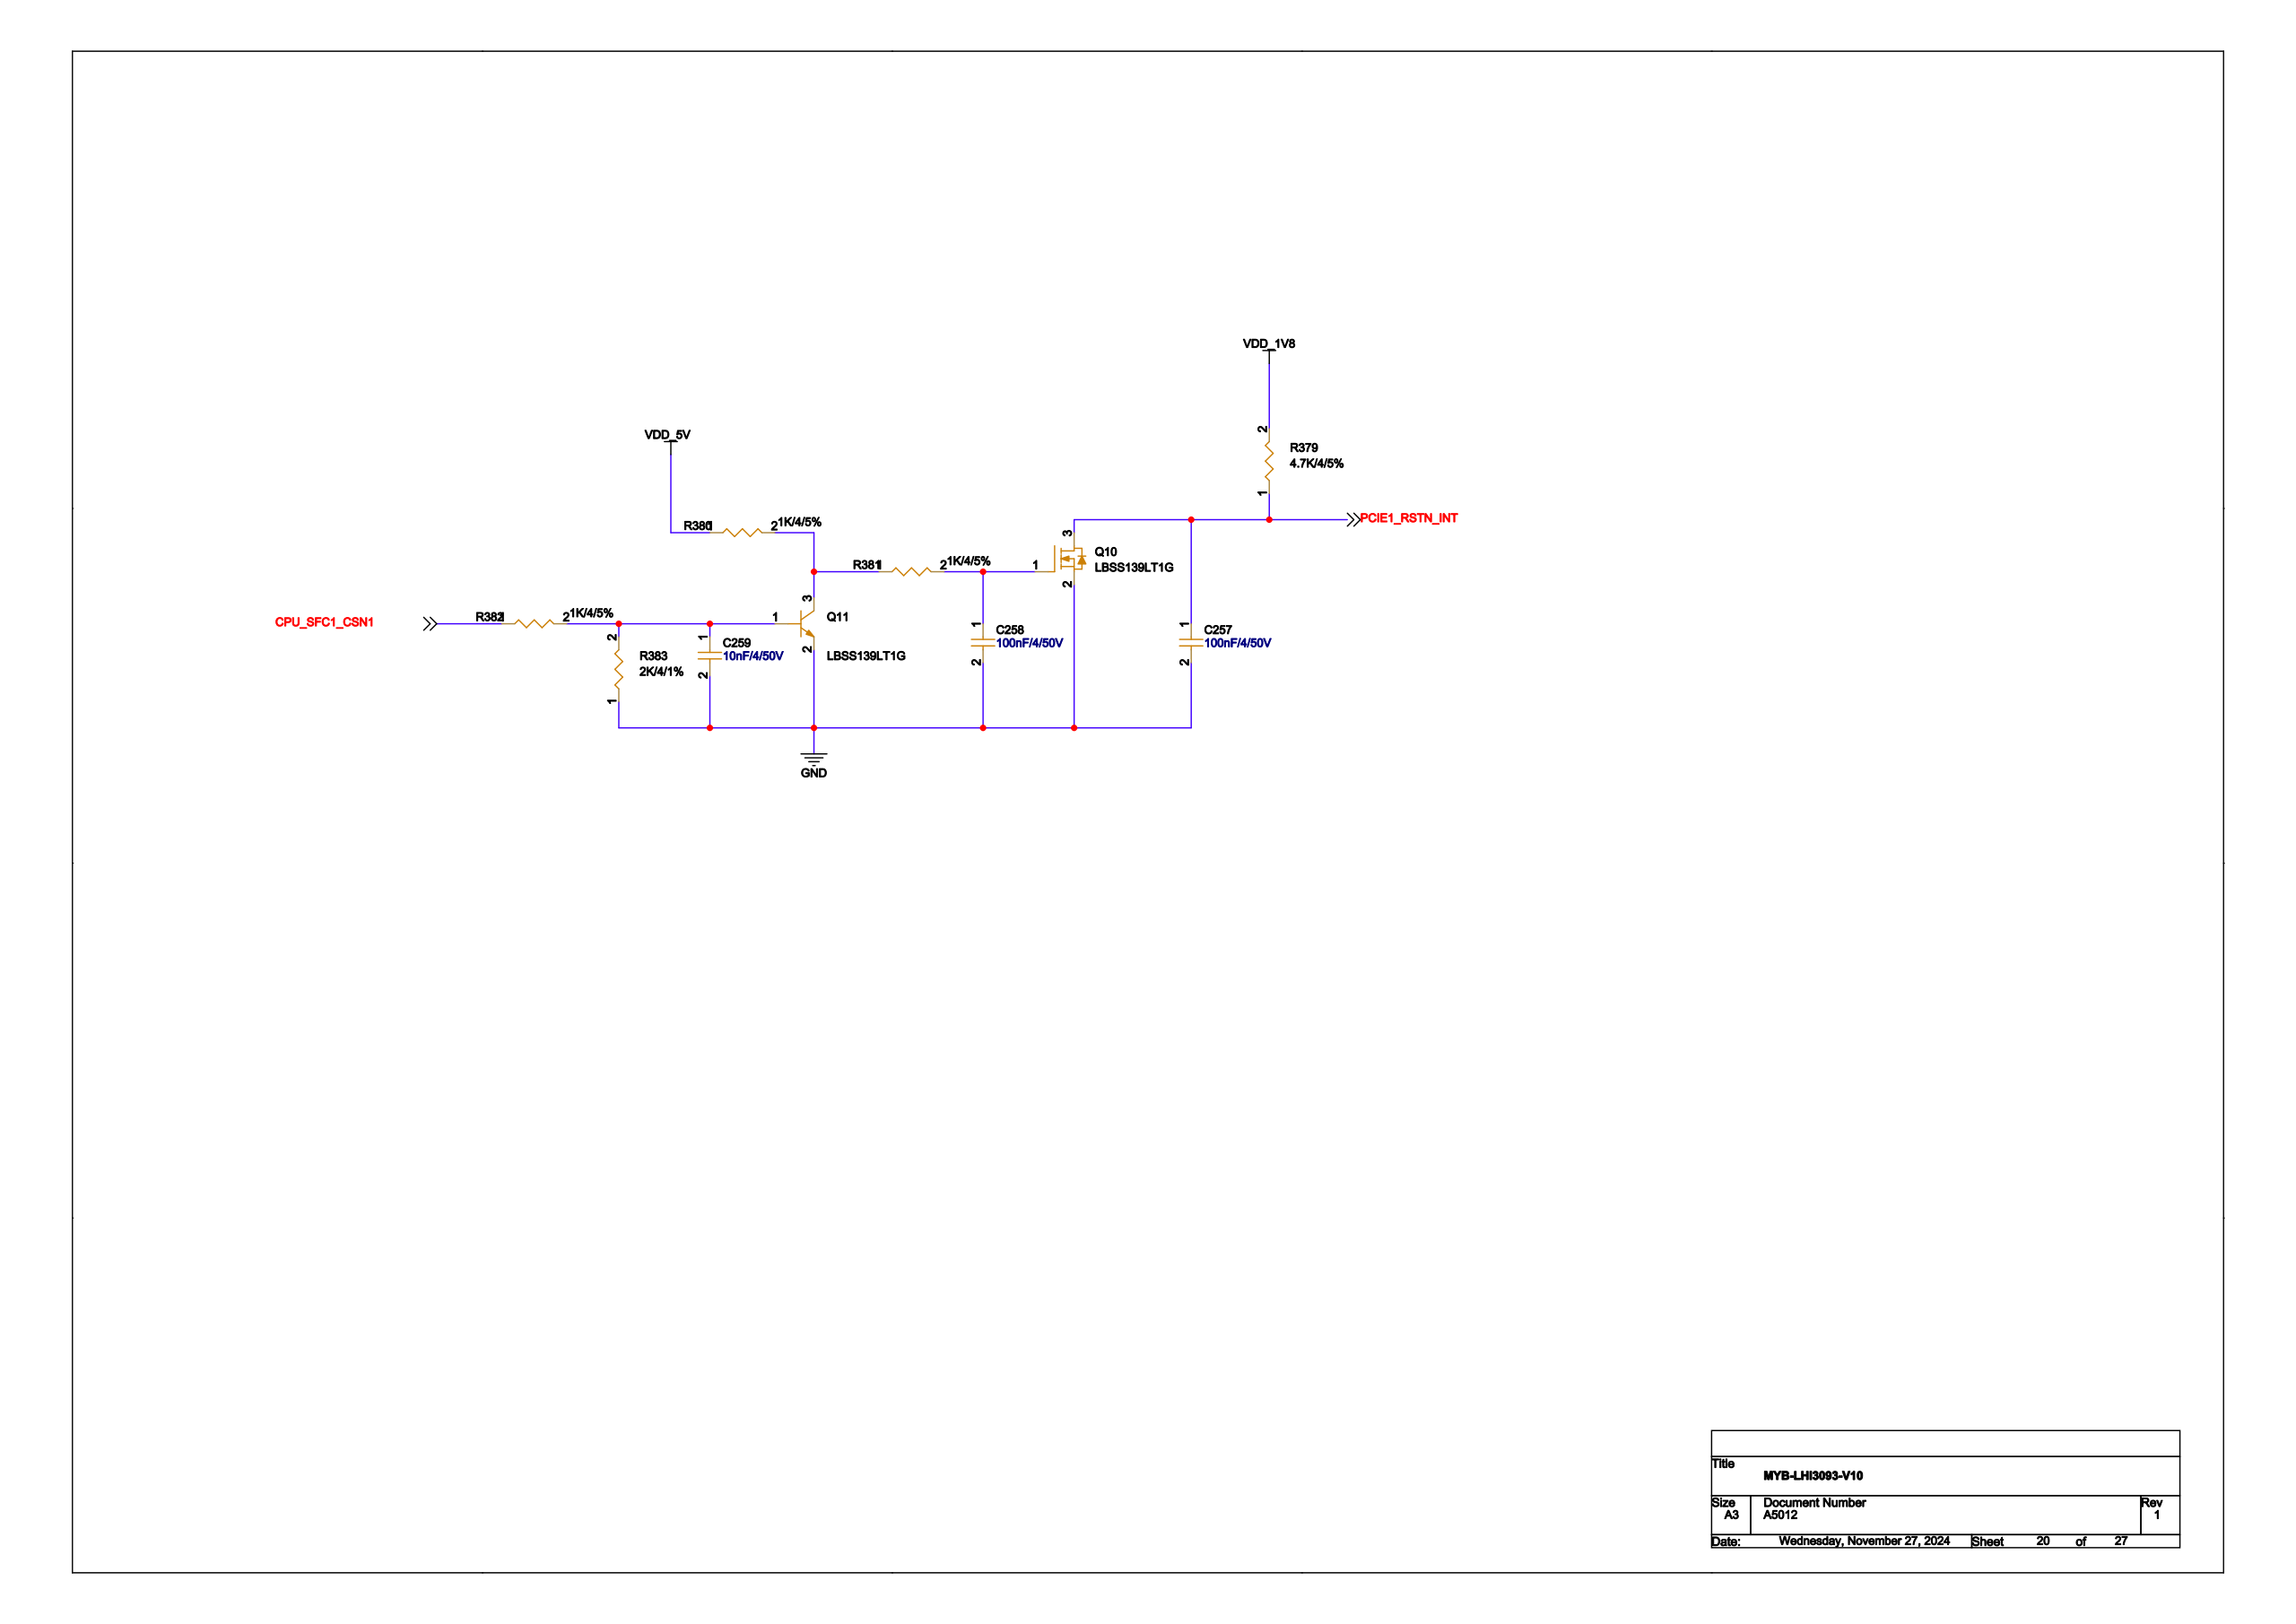Circuit board | Cadence Allegro | 1159 parts | 708 nets | one sheet of the schematic
Parts on this sheet (reference | value | footprint):
C257 | 100nF/4/50V | C0402
C258 | 100nF/4/50V | C0402
C259 | 10nF/4/50V | C0402
Q10 | LBSS139LT1G | SOT-23
Q11 | LBSS139LT1G | SOT-23
R379 | 4.7K/4/5% | R0402
R383 | 2K/4/1% | R0402
Nets of these parts (net: part-pin ...):
GND: C257-2 C258-2 C259-2 Q10-2 Q11-2 R383-1
VDD_1V8: R379-2
PCIE1_RSTN_INT: C257-1 Q10-3 R379-1
N15048618: C258-1 Q10-1
N15048874: C259-1 Q11-1 R383-2
N15048563: Q11-3